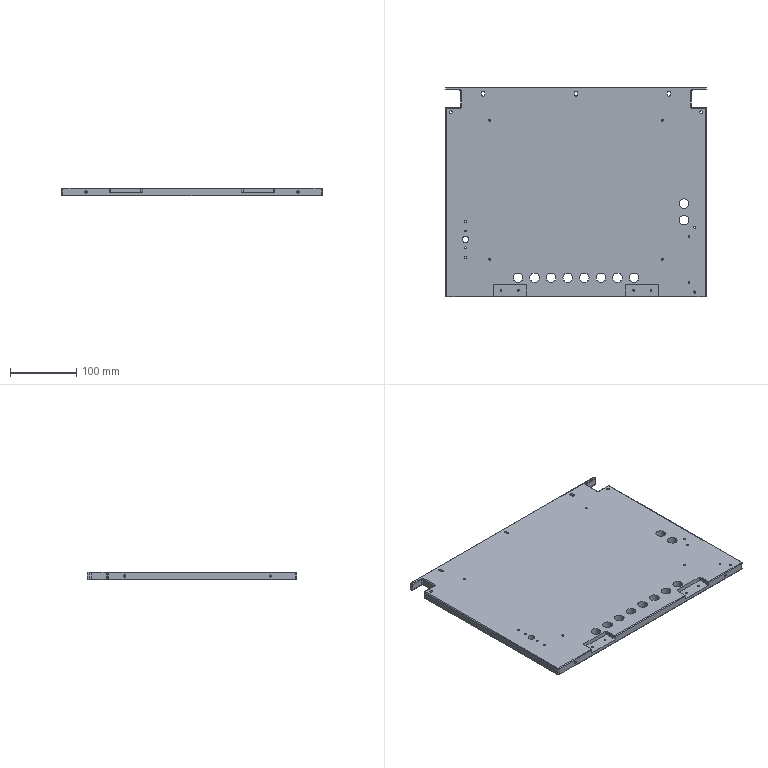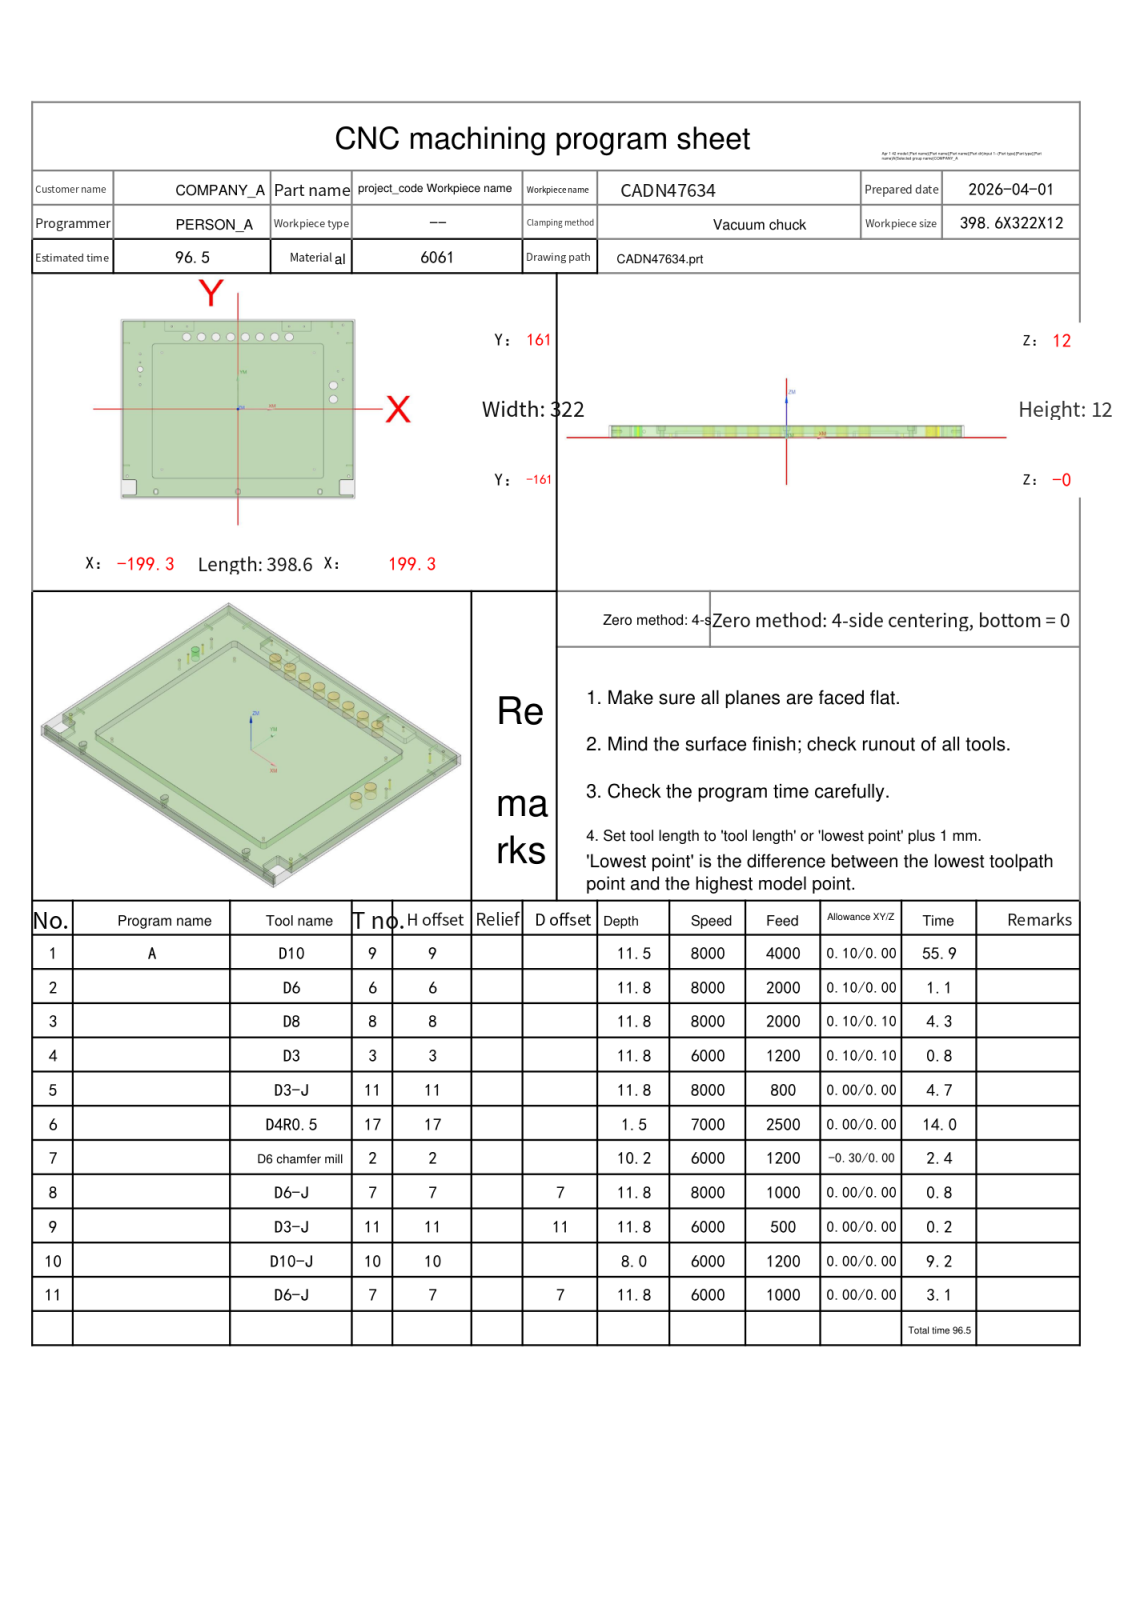NC program | NX | posted by the shop | part box 393.6 x 317 x 12 mm
Lines 3048 to 3819 of 16012:
N3 T08 M06
(D8  D=8. R=0. H=08 ce=0.10 di=0.10)
G00 G90 G54 X165.838 Y18.299 M03 S8000
G43 H08 Z32.
M08
Z13.
G01 X165.647 Y18.916 Z12.966 F2000.
X165.049 Y19.749 Z12.912
X164.216 Y20.347 Z12.859
X163.236 Y20.65 Z12.805
X162.364 Z12.759
X161.384 Y20.347 Z12.705
X160.551 Y19.749 Z12.652
X159.953 Y18.916 Z12.598
X159.65 Y17.936 Z12.544
Y17.5 Z12.521
Y17.064 Z12.499
X159.953 Y16.084 Z12.445
X160.551 Y15.251 Z12.391
X161.384 Y14.653 Z12.337
X162.364 Y14.35 Z12.284
X163.236 Z12.238
X164.216 Y14.653 Z12.184
X165.049 Y15.251 Z12.13
X165.647 Y16.084 Z12.077
X165.95 Y17.064 Z12.023
Y17.5 Z12.
G03 X162.8 Y20.65 Z11.926 I-3.15 J0.0
X159.65 Y17.5 Z11.853 I0.0 J-3.15
X162.8 Y14.35 Z11.779 I3.15 J0.0
X165.95 Y17.5 Z11.705 I0.0 J3.15
X162.8 Y20.65 Z11.631 I-3.15 J0.0
X159.65 Y17.5 Z11.558 I0.0 J-3.15
X162.8 Y14.35 Z11.484 I3.15 J0.0
X165.95 Y17.5 Z11.41 I0.0 J3.15
X162.8 Y20.65 Z11.336 I-3.15 J0.0
X159.65 Y17.5 Z11.263 I0.0 J-3.15
X162.8 Y14.35 Z11.189 I3.15 J0.0
X165.95 Y17.5 Z11.115 I0.0 J3.15
X162.8 Y20.65 Z11.041 I-3.15 J0.0
X159.65 Y17.5 Z10.968 I0.0 J-3.15
X162.8 Y14.35 Z10.894 I3.15 J0.0
X165.95 Y17.5 Z10.82 I0.0 J3.15
X162.8 Y20.65 Z10.746 I-3.15 J0.0
X159.65 Y17.5 Z10.673 I0.0 J-3.15
X162.8 Y14.35 Z10.599 I3.15 J0.0
X165.95 Y17.5 Z10.525 I0.0 J3.15
X162.8 Y20.65 Z10.451 I-3.15 J0.0
X159.65 Y17.5 Z10.378 I0.0 J-3.15
X162.8 Y14.35 Z10.304 I3.15 J0.0
X165.95 Y17.5 Z10.23 I0.0 J3.15
X162.8 Y20.65 Z10.156 I-3.15 J0.0
X159.65 Y17.5 Z10.083 I0.0 J-3.15
X162.8 Y14.35 Z10.009 I3.15 J0.0
X165.95 Y17.5 Z9.935 I0.0 J3.15
X162.8 Y20.65 Z9.861 I-3.15 J0.0
X159.65 Y17.5 Z9.788 I0.0 J-3.15
X162.8 Y14.35 Z9.714 I3.15 J0.0
X165.95 Y17.5 Z9.64 I0.0 J3.15
X162.8 Y20.65 Z9.566 I-3.15 J0.0
X159.65 Y17.5 Z9.493 I0.0 J-3.15
X162.8 Y14.35 Z9.419 I3.15 J0.0
X165.95 Y17.5 Z9.345 I0.0 J3.15
X162.8 Y20.65 Z9.271 I-3.15 J0.0
X159.65 Y17.5 Z9.198 I0.0 J-3.15
X162.8 Y14.35 Z9.124 I3.15 J0.0
X165.95 Y17.5 Z9.05 I0.0 J3.15
X162.8 Y20.65 Z8.976 I-3.15 J0.0
X159.65 Y17.5 Z8.903 I0.0 J-3.15
X162.8 Y14.35 Z8.829 I3.15 J0.0
X165.95 Y17.5 Z8.755 I0.0 J3.15
X162.8 Y20.65 Z8.681 I-3.15 J0.0
X159.65 Y17.5 Z8.608 I0.0 J-3.15
X162.8 Y14.35 Z8.534 I3.15 J0.0
X165.95 Y17.5 Z8.46 I0.0 J3.15
X162.8 Y20.65 Z8.386 I-3.15 J0.0
X159.65 Y17.5 Z8.313 I0.0 J-3.15
X162.8 Y14.35 Z8.239 I3.15 J0.0
X165.95 Y17.5 Z8.165 I0.0 J3.15
X162.8 Y20.65 Z8.091 I-3.15 J0.0
X159.65 Y17.5 Z8.018 I0.0 J-3.15
X162.8 Y14.35 Z7.944 I3.15 J0.0
X165.95 Y17.5 Z7.87 I0.0 J3.15
X162.8 Y20.65 Z7.796 I-3.15 J0.0
X159.65 Y17.5 Z7.723 I0.0 J-3.15
X162.8 Y14.35 Z7.649 I3.15 J0.0
X165.95 Y17.5 Z7.575 I0.0 J3.15
X162.8 Y20.65 Z7.501 I-3.15 J0.0
X159.65 Y17.5 Z7.428 I0.0 J-3.15
X162.8 Y14.35 Z7.354 I3.15 J0.0
X165.95 Y17.5 Z7.28 I0.0 J3.15
X162.8 Y20.65 Z7.206 I-3.15 J0.0
X159.65 Y17.5 Z7.133 I0.0 J-3.15
X162.8 Y14.35 Z7.059 I3.15 J0.0
X165.95 Y17.5 Z6.985 I0.0 J3.15
X162.8 Y20.65 Z6.911 I-3.15 J0.0
X159.65 Y17.5 Z6.838 I0.0 J-3.15
X162.8 Y14.35 Z6.764 I3.15 J0.0
X165.95 Y17.5 Z6.69 I0.0 J3.15
X162.8 Y20.65 Z6.616 I-3.15 J0.0
X159.65 Y17.5 Z6.543 I0.0 J-3.15
X162.8 Y14.35 Z6.469 I3.15 J0.0
X165.95 Y17.5 Z6.395 I0.0 J3.15
X162.8 Y20.65 Z6.321 I-3.15 J0.0
X159.65 Y17.5 Z6.248 I0.0 J-3.15
X162.8 Y14.35 Z6.174 I3.15 J0.0
X165.95 Y17.5 Z6.1 I0.0 J3.15
X162.8 Y20.65 Z6.026 I-3.15 J0.0
X159.65 Y17.5 Z5.953 I0.0 J-3.15
X162.8 Y14.35 Z5.879 I3.15 J0.0
X165.95 Y17.5 Z5.805 I0.0 J3.15
X162.8 Y20.65 Z5.731 I-3.15 J0.0
X159.65 Y17.5 Z5.658 I0.0 J-3.15
X162.8 Y14.35 Z5.584 I3.15 J0.0
X165.95 Y17.5 Z5.51 I0.0 J3.15
X162.8 Y20.65 Z5.436 I-3.15 J0.0
X159.65 Y17.5 Z5.363 I0.0 J-3.15
X162.8 Y14.35 Z5.289 I3.15 J0.0
X165.95 Y17.5 Z5.215 I0.0 J3.15
X162.8 Y20.65 Z5.141 I-3.15 J0.0
X159.65 Y17.5 Z5.068 I0.0 J-3.15
X162.8 Y14.35 Z4.994 I3.15 J0.0
X165.95 Y17.5 Z4.92 I0.0 J3.15
X162.8 Y20.65 Z4.846 I-3.15 J0.0
X159.65 Y17.5 Z4.773 I0.0 J-3.15
X162.8 Y14.35 Z4.699 I3.15 J0.0
X165.95 Y17.5 Z4.625 I0.0 J3.15
X162.8 Y20.65 Z4.551 I-3.15 J0.0
X159.65 Y17.5 Z4.478 I0.0 J-3.15
X162.8 Y14.35 Z4.404 I3.15 J0.0
X165.95 Y17.5 Z4.33 I0.0 J3.15
X162.8 Y20.65 Z4.256 I-3.15 J0.0
X159.65 Y17.5 Z4.183 I0.0 J-3.15
X162.8 Y14.35 Z4.109 I3.15 J0.0
X165.95 Y17.5 Z4.035 I0.0 J3.15
X162.8 Y20.65 Z3.961 I-3.15 J0.0
X159.65 Y17.5 Z3.888 I0.0 J-3.15
X162.8 Y14.35 Z3.814 I3.15 J0.0
X165.95 Y17.5 Z3.74 I0.0 J3.15
X162.8 Y20.65 Z3.666 I-3.15 J0.0
X159.65 Y17.5 Z3.593 I0.0 J-3.15
X162.8 Y14.35 Z3.519 I3.15 J0.0
X165.95 Y17.5 Z3.445 I0.0 J3.15
X162.8 Y20.65 Z3.371 I-3.15 J0.0
X159.65 Y17.5 Z3.298 I0.0 J-3.15
X162.8 Y14.35 Z3.224 I3.15 J0.0
X165.95 Y17.5 Z3.15 I0.0 J3.15
X162.8 Y20.65 Z3.076 I-3.15 J0.0
X159.65 Y17.5 Z3.003 I0.0 J-3.15
X162.8 Y14.35 Z2.929 I3.15 J0.0
X165.95 Y17.5 Z2.855 I0.0 J3.15
X162.8 Y20.65 Z2.781 I-3.15 J0.0
X159.65 Y17.5 Z2.708 I0.0 J-3.15
X162.8 Y14.35 Z2.634 I3.15 J0.0
X165.95 Y17.5 Z2.56 I0.0 J3.15
X162.8 Y20.65 Z2.486 I-3.15 J0.0
X159.65 Y17.5 Z2.413 I0.0 J-3.15
X162.8 Y14.35 Z2.339 I3.15 J0.0
X165.95 Y17.5 Z2.265 I0.0 J3.15
X162.8 Y20.65 Z2.191 I-3.15 J0.0
X159.65 Y17.5 Z2.118 I0.0 J-3.15
X162.8 Y14.35 Z2.044 I3.15 J0.0
X165.95 Y17.5 Z1.97 I0.0 J3.15
X162.8 Y20.65 Z1.896 I-3.15 J0.0
X159.65 Y17.5 Z1.823 I0.0 J-3.15
X162.8 Y14.35 Z1.749 I3.15 J0.0
X165.95 Y17.5 Z1.675 I0.0 J3.15
X162.8 Y20.65 Z1.601 I-3.15 J0.0
X159.65 Y17.5 Z1.528 I0.0 J-3.15
X162.8 Y14.35 Z1.454 I3.15 J0.0
X165.95 Y17.5 Z1.38 I0.0 J3.15
X162.8 Y20.65 Z1.306 I-3.15 J0.0
X159.65 Y17.5 Z1.233 I0.0 J-3.15
X162.8 Y14.35 Z1.159 I3.15 J0.0
X165.95 Y17.5 Z1.085 I0.0 J3.15
X162.8 Y20.65 Z1.011 I-3.15 J0.0
X159.65 Y17.5 Z.938 I0.0 J-3.15
X162.8 Y14.35 Z.864 I3.15 J0.0
X165.95 Y17.5 Z.79 I0.0 J3.15
X162.8 Y20.65 Z.716 I-3.15 J0.0
X159.65 Y17.5 Z.643 I0.0 J-3.15
X162.8 Y14.35 Z.569 I3.15 J0.0
X165.95 Y17.5 Z.495 I0.0 J3.15
X162.8 Y20.65 Z.421 I-3.15 J0.0
X159.65 Y17.5 Z.348 I0.0 J-3.15
X162.8 Y14.35 Z.274 I3.15 J0.0
X165.95 Y17.5 Z.2 I0.0 J3.15
X162.8 Y20.65 I-3.15 J0.0
X159.65 Y17.5 I0.0 J-3.15
X162.8 Y14.35 I3.15 J0.0
X165.95 Y17.5 I0.0 J3.15
X165.925 Y17.899 I-3.15 J0.0
G01 Z1.2
G00 Z32.
X165.838 Y43.299
Z13.
G01 X165.647 Y43.916 Z12.966
X165.049 Y44.749 Z12.912
X164.216 Y45.347 Z12.859
X163.236 Y45.65 Z12.805
X162.364 Z12.759
X161.384 Y45.347 Z12.705
X160.551 Y44.749 Z12.652
X159.953 Y43.916 Z12.598
X159.65 Y42.936 Z12.544
Y42.064 Z12.499
X159.953 Y41.084 Z12.445
X160.551 Y40.251 Z12.391
X161.384 Y39.653 Z12.337
X162.364 Y39.35 Z12.284
X163.236 Z12.238
X164.216 Y39.653 Z12.184
X165.049 Y40.251 Z12.13
X165.647 Y41.084 Z12.077
X165.95 Y42.064 Z12.023
Y42.5 Z12.
G03 X162.8 Y45.65 Z11.926 I-3.15 J0.0
X159.65 Y42.5 Z11.853 I0.0 J-3.15
X162.8 Y39.35 Z11.779 I3.15 J0.0
X165.95 Y42.5 Z11.705 I0.0 J3.15
X162.8 Y45.65 Z11.631 I-3.15 J0.0
X159.65 Y42.5 Z11.558 I0.0 J-3.15
X162.8 Y39.35 Z11.484 I3.15 J0.0
X165.95 Y42.5 Z11.41 I0.0 J3.15
X162.8 Y45.65 Z11.336 I-3.15 J0.0
X159.65 Y42.5 Z11.263 I0.0 J-3.15
X162.8 Y39.35 Z11.189 I3.15 J0.0
X165.95 Y42.5 Z11.115 I0.0 J3.15
X162.8 Y45.65 Z11.041 I-3.15 J0.0
X159.65 Y42.5 Z10.968 I0.0 J-3.15
X162.8 Y39.35 Z10.894 I3.15 J0.0
X165.95 Y42.5 Z10.82 I0.0 J3.15
X162.8 Y45.65 Z10.746 I-3.15 J0.0
X159.65 Y42.5 Z10.673 I0.0 J-3.15
X162.8 Y39.35 Z10.599 I3.15 J0.0
X165.95 Y42.5 Z10.525 I0.0 J3.15
X162.8 Y45.65 Z10.451 I-3.15 J0.0
X159.65 Y42.5 Z10.378 I0.0 J-3.15
X162.8 Y39.35 Z10.304 I3.15 J0.0
X165.95 Y42.5 Z10.23 I0.0 J3.15
X162.8 Y45.65 Z10.156 I-3.15 J0.0
X159.65 Y42.5 Z10.083 I0.0 J-3.15
X162.8 Y39.35 Z10.009 I3.15 J0.0
X165.95 Y42.5 Z9.935 I0.0 J3.15
X162.8 Y45.65 Z9.861 I-3.15 J0.0
X159.65 Y42.5 Z9.788 I0.0 J-3.15
X162.8 Y39.35 Z9.714 I3.15 J0.0
X165.95 Y42.5 Z9.64 I0.0 J3.15
X162.8 Y45.65 Z9.566 I-3.15 J0.0
X159.65 Y42.5 Z9.493 I0.0 J-3.15
X162.8 Y39.35 Z9.419 I3.15 J0.0
X165.95 Y42.5 Z9.345 I0.0 J3.15
X162.8 Y45.65 Z9.271 I-3.15 J0.0
X159.65 Y42.5 Z9.198 I0.0 J-3.15
X162.8 Y39.35 Z9.124 I3.15 J0.0
X165.95 Y42.5 Z9.05 I0.0 J3.15
X162.8 Y45.65 Z8.976 I-3.15 J0.0
X159.65 Y42.5 Z8.903 I0.0 J-3.15
X162.8 Y39.35 Z8.829 I3.15 J0.0
X165.95 Y42.5 Z8.755 I0.0 J3.15
X162.8 Y45.65 Z8.681 I-3.15 J0.0
X159.65 Y42.5 Z8.608 I0.0 J-3.15
X162.8 Y39.35 Z8.534 I3.15 J0.0
X165.95 Y42.5 Z8.46 I0.0 J3.15
X162.8 Y45.65 Z8.386 I-3.15 J0.0
X159.65 Y42.5 Z8.313 I0.0 J-3.15
X162.8 Y39.35 Z8.239 I3.15 J0.0
X165.95 Y42.5 Z8.165 I0.0 J3.15
X162.8 Y45.65 Z8.091 I-3.15 J0.0
X159.65 Y42.5 Z8.018 I0.0 J-3.15
X162.8 Y39.35 Z7.944 I3.15 J0.0
X165.95 Y42.5 Z7.87 I0.0 J3.15
X162.8 Y45.65 Z7.796 I-3.15 J0.0
X159.65 Y42.5 Z7.723 I0.0 J-3.15
X162.8 Y39.35 Z7.649 I3.15 J0.0
X165.95 Y42.5 Z7.575 I0.0 J3.15
X162.8 Y45.65 Z7.501 I-3.15 J0.0
X159.65 Y42.5 Z7.428 I0.0 J-3.15
X162.8 Y39.35 Z7.354 I3.15 J0.0
X165.95 Y42.5 Z7.28 I0.0 J3.15
X162.8 Y45.65 Z7.206 I-3.15 J0.0
X159.65 Y42.5 Z7.133 I0.0 J-3.15
X162.8 Y39.35 Z7.059 I3.15 J0.0
X165.95 Y42.5 Z6.985 I0.0 J3.15
X162.8 Y45.65 Z6.911 I-3.15 J0.0
X159.65 Y42.5 Z6.838 I0.0 J-3.15
X162.8 Y39.35 Z6.764 I3.15 J0.0
X165.95 Y42.5 Z6.69 I0.0 J3.15
X162.8 Y45.65 Z6.616 I-3.15 J0.0
X159.65 Y42.5 Z6.543 I0.0 J-3.15
X162.8 Y39.35 Z6.469 I3.15 J0.0
X165.95 Y42.5 Z6.395 I0.0 J3.15
X162.8 Y45.65 Z6.321 I-3.15 J0.0
X159.65 Y42.5 Z6.248 I0.0 J-3.15
X162.8 Y39.35 Z6.174 I3.15 J0.0
X165.95 Y42.5 Z6.1 I0.0 J3.15
X162.8 Y45.65 Z6.026 I-3.15 J0.0
X159.65 Y42.5 Z5.953 I0.0 J-3.15
X162.8 Y39.35 Z5.879 I3.15 J0.0
X165.95 Y42.5 Z5.805 I0.0 J3.15
X162.8 Y45.65 Z5.731 I-3.15 J0.0
X159.65 Y42.5 Z5.658 I0.0 J-3.15
X162.8 Y39.35 Z5.584 I3.15 J0.0
X165.95 Y42.5 Z5.51 I0.0 J3.15
X162.8 Y45.65 Z5.436 I-3.15 J0.0
X159.65 Y42.5 Z5.363 I0.0 J-3.15
X162.8 Y39.35 Z5.289 I3.15 J0.0
X165.95 Y42.5 Z5.215 I0.0 J3.15
X162.8 Y45.65 Z5.141 I-3.15 J0.0
X159.65 Y42.5 Z5.068 I0.0 J-3.15
X162.8 Y39.35 Z4.994 I3.15 J0.0
X165.95 Y42.5 Z4.92 I0.0 J3.15
X162.8 Y45.65 Z4.846 I-3.15 J0.0
X159.65 Y42.5 Z4.773 I0.0 J-3.15
X162.8 Y39.35 Z4.699 I3.15 J0.0
X165.95 Y42.5 Z4.625 I0.0 J3.15
X162.8 Y45.65 Z4.551 I-3.15 J0.0
X159.65 Y42.5 Z4.478 I0.0 J-3.15
X162.8 Y39.35 Z4.404 I3.15 J0.0
X165.95 Y42.5 Z4.33 I0.0 J3.15
X162.8 Y45.65 Z4.256 I-3.15 J0.0
X159.65 Y42.5 Z4.183 I0.0 J-3.15
X162.8 Y39.35 Z4.109 I3.15 J0.0
X165.95 Y42.5 Z4.035 I0.0 J3.15
X162.8 Y45.65 Z3.961 I-3.15 J0.0
X159.65 Y42.5 Z3.888 I0.0 J-3.15
X162.8 Y39.35 Z3.814 I3.15 J0.0
X165.95 Y42.5 Z3.74 I0.0 J3.15
X162.8 Y45.65 Z3.666 I-3.15 J0.0
X159.65 Y42.5 Z3.593 I0.0 J-3.15
X162.8 Y39.35 Z3.519 I3.15 J0.0
X165.95 Y42.5 Z3.445 I0.0 J3.15
X162.8 Y45.65 Z3.371 I-3.15 J0.0
X159.65 Y42.5 Z3.298 I0.0 J-3.15
X162.8 Y39.35 Z3.224 I3.15 J0.0
X165.95 Y42.5 Z3.15 I0.0 J3.15
X162.8 Y45.65 Z3.076 I-3.15 J0.0
X159.65 Y42.5 Z3.003 I0.0 J-3.15
X162.8 Y39.35 Z2.929 I3.15 J0.0
X165.95 Y42.5 Z2.855 I0.0 J3.15
X162.8 Y45.65 Z2.781 I-3.15 J0.0
X159.65 Y42.5 Z2.708 I0.0 J-3.15
X162.8 Y39.35 Z2.634 I3.15 J0.0
X165.95 Y42.5 Z2.56 I0.0 J3.15
X162.8 Y45.65 Z2.486 I-3.15 J0.0
X159.65 Y42.5 Z2.413 I0.0 J-3.15
X162.8 Y39.35 Z2.339 I3.15 J0.0
X165.95 Y42.5 Z2.265 I0.0 J3.15
X162.8 Y45.65 Z2.191 I-3.15 J0.0
X159.65 Y42.5 Z2.118 I0.0 J-3.15
X162.8 Y39.35 Z2.044 I3.15 J0.0
X165.95 Y42.5 Z1.97 I0.0 J3.15
X162.8 Y45.65 Z1.896 I-3.15 J0.0
X159.65 Y42.5 Z1.823 I0.0 J-3.15
X162.8 Y39.35 Z1.749 I3.15 J0.0
X165.95 Y42.5 Z1.675 I0.0 J3.15
X162.8 Y45.65 Z1.601 I-3.15 J0.0
X159.65 Y42.5 Z1.528 I0.0 J-3.15
X162.8 Y39.35 Z1.454 I3.15 J0.0
X165.95 Y42.5 Z1.38 I0.0 J3.15
X162.8 Y45.65 Z1.306 I-3.15 J0.0
X159.65 Y42.5 Z1.233 I0.0 J-3.15
X162.8 Y39.35 Z1.159 I3.15 J0.0
X165.95 Y42.5 Z1.085 I0.0 J3.15
X162.8 Y45.65 Z1.011 I-3.15 J0.0
X159.65 Y42.5 Z.938 I0.0 J-3.15
X162.8 Y39.35 Z.864 I3.15 J0.0
X165.95 Y42.5 Z.79 I0.0 J3.15
X162.8 Y45.65 Z.716 I-3.15 J0.0
X159.65 Y42.5 Z.643 I0.0 J-3.15
X162.8 Y39.35 Z.569 I3.15 J0.0
X165.95 Y42.5 Z.495 I0.0 J3.15
X162.8 Y45.65 Z.421 I-3.15 J0.0
X159.65 Y42.5 Z.348 I0.0 J-3.15
X162.8 Y39.35 Z.274 I3.15 J0.0
X165.95 Y42.5 Z.2 I0.0 J3.15
X162.8 Y45.65 I-3.15 J0.0
X159.65 Y42.5 I0.0 J-3.15
X162.8 Y39.35 I3.15 J0.0
X165.95 Y42.5 I0.0 J3.15
X165.925 Y42.899 I-3.15 J0.0
G01 Z1.2
G00 Z32.
X-88.299 Y132.538
Z13.
G01 X-88.916 Y132.347 Z12.966
X-89.749 Y131.749 Z12.912
X-90.347 Y130.916 Z12.859
X-90.65 Y129.936 Z12.805
Y129.5 Z12.782
Y129.064 Z12.759
X-90.347 Y128.084 Z12.705
X-89.749 Y127.251 Z12.652
X-88.916 Y126.653 Z12.598
X-87.936 Y126.35 Z12.544
X-87.064 Z12.499
X-86.084 Y126.653 Z12.445
X-85.251 Y127.251 Z12.391
X-84.653 Y128.084 Z12.337
X-84.35 Y129.064 Z12.284
Y129.936 Z12.238
X-84.653 Y130.916 Z12.184
X-85.251 Y131.749 Z12.13
X-86.084 Y132.347 Z12.077
X-87.064 Y132.65 Z12.023
X-87.5 Z12.
G03 X-90.65 Y129.5 Z11.926 I0.0 J-3.15
X-87.5 Y126.35 Z11.853 I3.15 J0.0
X-84.35 Y129.5 Z11.779 I0.0 J3.15
X-87.5 Y132.65 Z11.705 I-3.15 J0.0
X-90.65 Y129.5 Z11.631 I0.0 J-3.15
X-87.5 Y126.35 Z11.558 I3.15 J0.0
X-84.35 Y129.5 Z11.484 I0.0 J3.15
X-87.5 Y132.65 Z11.41 I-3.15 J0.0
X-90.65 Y129.5 Z11.336 I0.0 J-3.15
X-87.5 Y126.35 Z11.263 I3.15 J0.0
X-84.35 Y129.5 Z11.189 I0.0 J3.15
X-87.5 Y132.65 Z11.115 I-3.15 J0.0
X-90.65 Y129.5 Z11.041 I0.0 J-3.15
X-87.5 Y126.35 Z10.968 I3.15 J0.0
X-84.35 Y129.5 Z10.894 I0.0 J3.15
X-87.5 Y132.65 Z10.82 I-3.15 J0.0
X-90.65 Y129.5 Z10.746 I0.0 J-3.15
X-87.5 Y126.35 Z10.673 I3.15 J0.0
X-84.35 Y129.5 Z10.599 I0.0 J3.15
X-87.5 Y132.65 Z10.525 I-3.15 J0.0
X-90.65 Y129.5 Z10.451 I0.0 J-3.15
X-87.5 Y126.35 Z10.378 I3.15 J0.0
X-84.35 Y129.5 Z10.304 I0.0 J3.15
X-87.5 Y132.65 Z10.23 I-3.15 J0.0
X-90.65 Y129.5 Z10.156 I0.0 J-3.15
X-87.5 Y126.35 Z10.083 I3.15 J0.0
X-84.35 Y129.5 Z10.009 I0.0 J3.15
X-87.5 Y132.65 Z9.935 I-3.15 J0.0
X-90.65 Y129.5 Z9.861 I0.0 J-3.15
X-87.5 Y126.35 Z9.788 I3.15 J0.0
X-84.35 Y129.5 Z9.714 I0.0 J3.15
X-87.5 Y132.65 Z9.64 I-3.15 J0.0
X-90.65 Y129.5 Z9.566 I0.0 J-3.15
X-87.5 Y126.35 Z9.493 I3.15 J0.0
X-84.35 Y129.5 Z9.419 I0.0 J3.15
X-87.5 Y132.65 Z9.345 I-3.15 J0.0
X-90.65 Y129.5 Z9.271 I0.0 J-3.15
X-87.5 Y126.35 Z9.198 I3.15 J0.0
X-84.35 Y129.5 Z9.124 I0.0 J3.15
X-87.5 Y132.65 Z9.05 I-3.15 J0.0
X-90.65 Y129.5 Z8.976 I0.0 J-3.15
X-87.5 Y126.35 Z8.903 I3.15 J0.0
X-84.35 Y129.5 Z8.829 I0.0 J3.15
X-87.5 Y132.65 Z8.755 I-3.15 J0.0
X-90.65 Y129.5 Z8.681 I0.0 J-3.15
X-87.5 Y126.35 Z8.608 I3.15 J0.0
X-84.35 Y129.5 Z8.534 I0.0 J3.15
X-87.5 Y132.65 Z8.46 I-3.15 J0.0
X-90.65 Y129.5 Z8.386 I0.0 J-3.15
X-87.5 Y126.35 Z8.313 I3.15 J0.0
X-84.35 Y129.5 Z8.239 I0.0 J3.15
X-87.5 Y132.65 Z8.165 I-3.15 J0.0
X-90.65 Y129.5 Z8.091 I0.0 J-3.15
X-87.5 Y126.35 Z8.018 I3.15 J0.0
X-84.35 Y129.5 Z7.944 I0.0 J3.15
X-87.5 Y132.65 Z7.87 I-3.15 J0.0
X-90.65 Y129.5 Z7.796 I0.0 J-3.15
X-87.5 Y126.35 Z7.723 I3.15 J0.0
X-84.35 Y129.5 Z7.649 I0.0 J3.15
X-87.5 Y132.65 Z7.575 I-3.15 J0.0
X-90.65 Y129.5 Z7.501 I0.0 J-3.15
X-87.5 Y126.35 Z7.428 I3.15 J0.0
X-84.35 Y129.5 Z7.354 I0.0 J3.15
X-87.5 Y132.65 Z7.28 I-3.15 J0.0
X-90.65 Y129.5 Z7.206 I0.0 J-3.15
X-87.5 Y126.35 Z7.133 I3.15 J0.0
X-84.35 Y129.5 Z7.059 I0.0 J3.15
X-87.5 Y132.65 Z6.985 I-3.15 J0.0
X-90.65 Y129.5 Z6.911 I0.0 J-3.15
X-87.5 Y126.35 Z6.838 I3.15 J0.0
X-84.35 Y129.5 Z6.764 I0.0 J3.15
X-87.5 Y132.65 Z6.69 I-3.15 J0.0
X-90.65 Y129.5 Z6.616 I0.0 J-3.15
X-87.5 Y126.35 Z6.543 I3.15 J0.0
X-84.35 Y129.5 Z6.469 I0.0 J3.15
X-87.5 Y132.65 Z6.395 I-3.15 J0.0
X-90.65 Y129.5 Z6.321 I0.0 J-3.15
X-87.5 Y126.35 Z6.248 I3.15 J0.0
X-84.35 Y129.5 Z6.174 I0.0 J3.15
X-87.5 Y132.65 Z6.1 I-3.15 J0.0
X-90.65 Y129.5 Z6.026 I0.0 J-3.15
X-87.5 Y126.35 Z5.953 I3.15 J0.0
X-84.35 Y129.5 Z5.879 I0.0 J3.15
X-87.5 Y132.65 Z5.805 I-3.15 J0.0
X-90.65 Y129.5 Z5.731 I0.0 J-3.15
X-87.5 Y126.35 Z5.658 I3.15 J0.0
X-84.35 Y129.5 Z5.584 I0.0 J3.15
X-87.5 Y132.65 Z5.51 I-3.15 J0.0
X-90.65 Y129.5 Z5.436 I0.0 J-3.15
X-87.5 Y126.35 Z5.363 I3.15 J0.0
X-84.35 Y129.5 Z5.289 I0.0 J3.15
X-87.5 Y132.65 Z5.215 I-3.15 J0.0
X-90.65 Y129.5 Z5.141 I0.0 J-3.15
X-87.5 Y126.35 Z5.068 I3.15 J0.0
X-84.35 Y129.5 Z4.994 I0.0 J3.15
X-87.5 Y132.65 Z4.92 I-3.15 J0.0
X-90.65 Y129.5 Z4.846 I0.0 J-3.15
X-87.5 Y126.35 Z4.773 I3.15 J0.0
X-84.35 Y129.5 Z4.699 I0.0 J3.15
X-87.5 Y132.65 Z4.625 I-3.15 J0.0
X-90.65 Y129.5 Z4.551 I0.0 J-3.15
X-87.5 Y126.35 Z4.478 I3.15 J0.0
X-84.35 Y129.5 Z4.404 I0.0 J3.15
X-87.5 Y132.65 Z4.33 I-3.15 J0.0
X-90.65 Y129.5 Z4.256 I0.0 J-3.15
X-87.5 Y126.35 Z4.183 I3.15 J0.0
X-84.35 Y129.5 Z4.109 I0.0 J3.15
X-87.5 Y132.65 Z4.035 I-3.15 J0.0
X-90.65 Y129.5 Z3.961 I0.0 J-3.15
X-87.5 Y126.35 Z3.888 I3.15 J0.0
X-84.35 Y129.5 Z3.814 I0.0 J3.15
X-87.5 Y132.65 Z3.74 I-3.15 J0.0
X-90.65 Y129.5 Z3.666 I0.0 J-3.15
X-87.5 Y126.35 Z3.593 I3.15 J0.0
X-84.35 Y129.5 Z3.519 I0.0 J3.15
X-87.5 Y132.65 Z3.445 I-3.15 J0.0
X-90.65 Y129.5 Z3.371 I0.0 J-3.15
X-87.5 Y126.35 Z3.298 I3.15 J0.0
X-84.35 Y129.5 Z3.224 I0.0 J3.15
X-87.5 Y132.65 Z3.15 I-3.15 J0.0
X-90.65 Y129.5 Z3.076 I0.0 J-3.15
X-87.5 Y126.35 Z3.003 I3.15 J0.0
X-84.35 Y129.5 Z2.929 I0.0 J3.15
X-87.5 Y132.65 Z2.855 I-3.15 J0.0
X-90.65 Y129.5 Z2.781 I0.0 J-3.15
X-87.5 Y126.35 Z2.708 I3.15 J0.0
X-84.35 Y129.5 Z2.634 I0.0 J3.15
X-87.5 Y132.65 Z2.56 I-3.15 J0.0
X-90.65 Y129.5 Z2.486 I0.0 J-3.15
X-87.5 Y126.35 Z2.413 I3.15 J0.0
X-84.35 Y129.5 Z2.339 I0.0 J3.15
X-87.5 Y132.65 Z2.265 I-3.15 J0.0
X-90.65 Y129.5 Z2.191 I0.0 J-3.15
X-87.5 Y126.35 Z2.118 I3.15 J0.0
X-84.35 Y129.5 Z2.044 I0.0 J3.15
X-87.5 Y132.65 Z1.97 I-3.15 J0.0
X-90.65 Y129.5 Z1.896 I0.0 J-3.15
X-87.5 Y126.35 Z1.823 I3.15 J0.0
X-84.35 Y129.5 Z1.749 I0.0 J3.15
X-87.5 Y132.65 Z1.675 I-3.15 J0.0
X-90.65 Y129.5 Z1.601 I0.0 J-3.15
X-87.5 Y126.35 Z1.528 I3.15 J0.0
X-84.35 Y129.5 Z1.454 I0.0 J3.15
X-87.5 Y132.65 Z1.38 I-3.15 J0.0
X-90.65 Y129.5 Z1.306 I0.0 J-3.15
X-87.5 Y126.35 Z1.233 I3.15 J0.0
X-84.35 Y129.5 Z1.159 I0.0 J3.15
X-87.5 Y132.65 Z1.085 I-3.15 J0.0
X-90.65 Y129.5 Z1.011 I0.0 J-3.15
X-87.5 Y126.35 Z.938 I3.15 J0.0
X-84.35 Y129.5 Z.864 I0.0 J3.15
X-87.5 Y132.65 Z.79 I-3.15 J0.0
X-90.65 Y129.5 Z.716 I0.0 J-3.15
X-87.5 Y126.35 Z.643 I3.15 J0.0
X-84.35 Y129.5 Z.569 I0.0 J3.15
X-87.5 Y132.65 Z.495 I-3.15 J0.0
X-90.65 Y129.5 Z.421 I0.0 J-3.15
X-87.5 Y126.35 Z.348 I3.15 J0.0
X-84.35 Y129.5 Z.274 I0.0 J3.15
X-87.5 Y132.65 Z.2 I-3.15 J0.0
X-90.65 Y129.5 I0.0 J-3.15
X-87.5 Y126.35 I3.15 J0.0
X-84.35 Y129.5 I0.0 J3.15
X-87.5 Y132.65 I-3.15 J0.0
X-87.899 Y132.625 I0.0 J-3.15
G01 Z1.2
G00 Z32.
X-63.299 Y132.538
Z13.
G01 X-63.916 Y132.347 Z12.966
X-64.749 Y131.749 Z12.912
X-65.347 Y130.916 Z12.859
X-65.65 Y129.936 Z12.805
Y129.5 Z12.782
Y129.064 Z12.759
X-65.347 Y128.084 Z12.705
X-64.749 Y127.251 Z12.652
X-63.916 Y126.653 Z12.598
X-62.936 Y126.35 Z12.544
X-62.5 Z12.521
X-62.064 Z12.499
X-61.084 Y126.653 Z12.445
X-60.251 Y127.251 Z12.391
X-59.653 Y128.084 Z12.337
X-59.35 Y129.064 Z12.284
Y129.5 Z12.261
Y129.936 Z12.238
X-59.653 Y130.916 Z12.184
X-60.251 Y131.749 Z12.13
X-61.084 Y132.347 Z12.077
X-62.064 Y132.65 Z12.023
X-62.5 Z12.
G03 X-65.65 Y129.5 Z11.926 I0.0 J-3.15
X-62.5 Y126.35 Z11.853 I3.15 J0.0
X-59.35 Y129.5 Z11.779 I0.0 J3.15
X-62.5 Y132.65 Z11.705 I-3.15 J0.0
X-65.65 Y129.5 Z11.631 I0.0 J-3.15
X-62.5 Y126.35 Z11.558 I3.15 J0.0
X-59.35 Y129.5 Z11.484 I0.0 J3.15
X-62.5 Y132.65 Z11.41 I-3.15 J0.0
X-65.65 Y129.5 Z11.336 I0.0 J-3.15
X-62.5 Y126.35 Z11.263 I3.15 J0.0
X-59.35 Y129.5 Z11.189 I0.0 J3.15
X-62.5 Y132.65 Z11.115 I-3.15 J0.0
X-65.65 Y129.5 Z11.041 I0.0 J-3.15
X-62.5 Y126.35 Z10.968 I3.15 J0.0
X-59.35 Y129.5 Z10.894 I0.0 J3.15
X-62.5 Y132.65 Z10.82 I-3.15 J0.0
X-65.65 Y129.5 Z10.746 I0.0 J-3.15
X-62.5 Y126.35 Z10.673 I3.15 J0.0
X-59.35 Y129.5 Z10.599 I0.0 J3.15
X-62.5 Y132.65 Z10.525 I-3.15 J0.0
X-65.65 Y129.5 Z10.451 I0.0 J-3.15
X-62.5 Y126.35 Z10.378 I3.15 J0.0
X-59.35 Y129.5 Z10.304 I0.0 J3.15
X-62.5 Y132.65 Z10.23 I-3.15 J0.0
X-65.65 Y129.5 Z10.156 I0.0 J-3.15
X-62.5 Y126.35 Z10.083 I3.15 J0.0
X-59.35 Y129.5 Z10.009 I0.0 J3.15
X-62.5 Y132.65 Z9.935 I-3.15 J0.0
X-65.65 Y129.5 Z9.861 I0.0 J-3.15
X-62.5 Y126.35 Z9.788 I3.15 J0.0
X-59.35 Y129.5 Z9.714 I0.0 J3.15
X-62.5 Y132.65 Z9.64 I-3.15 J0.0
X-65.65 Y129.5 Z9.566 I0.0 J-3.15
X-62.5 Y126.35 Z9.493 I3.15 J0.0
X-59.35 Y129.5 Z9.419 I0.0 J3.15
X-62.5 Y132.65 Z9.345 I-3.15 J0.0
X-65.65 Y129.5 Z9.271 I0.0 J-3.15
X-62.5 Y126.35 Z9.198 I3.15 J0.0
X-59.35 Y129.5 Z9.124 I0.0 J3.15
X-62.5 Y132.65 Z9.05 I-3.15 J0.0
X-65.65 Y129.5 Z8.976 I0.0 J-3.15
X-62.5 Y126.35 Z8.903 I3.15 J0.0
X-59.35 Y129.5 Z8.829 I0.0 J3.15
X-62.5 Y132.65 Z8.755 I-3.15 J0.0
X-65.65 Y129.5 Z8.681 I0.0 J-3.15
X-62.5 Y126.35 Z8.608 I3.15 J0.0
X-59.35 Y129.5 Z8.534 I0.0 J3.15
X-62.5 Y132.65 Z8.46 I-3.15 J0.0
X-65.65 Y129.5 Z8.386 I0.0 J-3.15
X-62.5 Y126.35 Z8.313 I3.15 J0.0
X-59.35 Y129.5 Z8.239 I0.0 J3.15
X-62.5 Y132.65 Z8.165 I-3.15 J0.0
X-65.65 Y129.5 Z8.091 I0.0 J-3.15
X-62.5 Y126.35 Z8.018 I3.15 J0.0
X-59.35 Y129.5 Z7.944 I0.0 J3.15
X-62.5 Y132.65 Z7.87 I-3.15 J0.0
X-65.65 Y129.5 Z7.796 I0.0 J-3.15
X-62.5 Y126.35 Z7.723 I3.15 J0.0
X-59.35 Y129.5 Z7.649 I0.0 J3.15
X-62.5 Y132.65 Z7.575 I-3.15 J0.0
X-65.65 Y129.5 Z7.501 I0.0 J-3.15
X-62.5 Y126.35 Z7.428 I3.15 J0.0
X-59.35 Y129.5 Z7.354 I0.0 J3.15
X-62.5 Y132.65 Z7.28 I-3.15 J0.0
X-65.65 Y129.5 Z7.206 I0.0 J-3.15
X-62.5 Y126.35 Z7.133 I3.15 J0.0
X-59.35 Y129.5 Z7.059 I0.0 J3.15
X-62.5 Y132.65 Z6.985 I-3.15 J0.0
X-65.65 Y129.5 Z6.911 I0.0 J-3.15
X-62.5 Y126.35 Z6.838 I3.15 J0.0
X-59.35 Y129.5 Z6.764 I0.0 J3.15
X-62.5 Y132.65 Z6.69 I-3.15 J0.0
X-65.65 Y129.5 Z6.616 I0.0 J-3.15
X-62.5 Y126.35 Z6.543 I3.15 J0.0
X-59.35 Y129.5 Z6.469 I0.0 J3.15
X-62.5 Y132.65 Z6.395 I-3.15 J0.0
X-65.65 Y129.5 Z6.321 I0.0 J-3.15
X-62.5 Y126.35 Z6.248 I3.15 J0.0
X-59.35 Y129.5 Z6.174 I0.0 J3.15
X-62.5 Y132.65 Z6.1 I-3.15 J0.0
X-65.65 Y129.5 Z6.026 I0.0 J-3.15
X-62.5 Y126.35 Z5.953 I3.15 J0.0
X-59.35 Y129.5 Z5.879 I0.0 J3.15
X-62.5 Y132.65 Z5.805 I-3.15 J0.0
X-65.65 Y129.5 Z5.731 I0.0 J-3.15
X-62.5 Y126.35 Z5.658 I3.15 J0.0
X-59.35 Y129.5 Z5.584 I0.0 J3.15
X-62.5 Y132.65 Z5.51 I-3.15 J0.0
X-65.65 Y129.5 Z5.436 I0.0 J-3.15
X-62.5 Y126.35 Z5.363 I3.15 J0.0
X-59.35 Y129.5 Z5.289 I0.0 J3.15
X-62.5 Y132.65 Z5.215 I-3.15 J0.0
X-65.65 Y129.5 Z5.141 I0.0 J-3.15
X-62.5 Y126.35 Z5.068 I3.15 J0.0
X-59.35 Y129.5 Z4.994 I0.0 J3.15
X-62.5 Y132.65 Z4.92 I-3.15 J0.0
X-65.65 Y129.5 Z4.846 I0.0 J-3.15
X-62.5 Y126.35 Z4.773 I3.15 J0.0
X-59.35 Y129.5 Z4.699 I0.0 J3.15
X-62.5 Y132.65 Z4.625 I-3.15 J0.0
X-65.65 Y129.5 Z4.551 I0.0 J-3.15
X-62.5 Y126.35 Z4.478 I3.15 J0.0
X-59.35 Y129.5 Z4.404 I0.0 J3.15
X-62.5 Y132.65 Z4.33 I-3.15 J0.0
X-65.65 Y129.5 Z4.256 I0.0 J-3.15
X-62.5 Y126.35 Z4.183 I3.15 J0.0
X-59.35 Y129.5 Z4.109 I0.0 J3.15
X-62.5 Y132.65 Z4.035 I-3.15 J0.0
X-65.65 Y129.5 Z3.961 I0.0 J-3.15
X-62.5 Y126.35 Z3.888 I3.15 J0.0
X-59.35 Y129.5 Z3.814 I0.0 J3.15
X-62.5 Y132.65 Z3.74 I-3.15 J0.0
X-65.65 Y129.5 Z3.666 I0.0 J-3.15
X-62.5 Y126.35 Z3.593 I3.15 J0.0
X-59.35 Y129.5 Z3.519 I0.0 J3.15
X-62.5 Y132.65 Z3.445 I-3.15 J0.0
X-65.65 Y129.5 Z3.371 I0.0 J-3.15
X-62.5 Y126.35 Z3.298 I3.15 J0.0
X-59.35 Y129.5 Z3.224 I0.0 J3.15
X-62.5 Y132.65 Z3.15 I-3.15 J0.0
X-65.65 Y129.5 Z3.076 I0.0 J-3.15
X-62.5 Y126.35 Z3.003 I3.15 J0.0
X-59.35 Y129.5 Z2.929 I0.0 J3.15
X-62.5 Y132.65 Z2.855 I-3.15 J0.0
X-65.65 Y129.5 Z2.781 I0.0 J-3.15
X-62.5 Y126.35 Z2.708 I3.15 J0.0
X-59.35 Y129.5 Z2.634 I0.0 J3.15
X-62.5 Y132.65 Z2.56 I-3.15 J0.0
X-65.65 Y129.5 Z2.486 I0.0 J-3.15
X-62.5 Y126.35 Z2.413 I3.15 J0.0
X-59.35 Y129.5 Z2.339 I0.0 J3.15
X-62.5 Y132.65 Z2.265 I-3.15 J0.0
X-65.65 Y129.5 Z2.191 I0.0 J-3.15
X-62.5 Y126.35 Z2.118 I3.15 J0.0
X-59.35 Y129.5 Z2.044 I0.0 J3.15
X-62.5 Y132.65 Z1.97 I-3.15 J0.0
X-65.65 Y129.5 Z1.896 I0.0 J-3.15
X-62.5 Y126.35 Z1.823 I3.15 J0.0
X-59.35 Y129.5 Z1.749 I0.0 J3.15
X-62.5 Y132.65 Z1.675 I-3.15 J0.0
X-65.65 Y129.5 Z1.601 I0.0 J-3.15
X-62.5 Y126.35 Z1.528 I3.15 J0.0
X-59.35 Y129.5 Z1.454 I0.0 J3.15
X-62.5 Y132.65 Z1.38 I-3.15 J0.0
X-65.65 Y129.5 Z1.306 I0.0 J-3.15
X-62.5 Y126.35 Z1.233 I3.15 J0.0
X-59.35 Y129.5 Z1.159 I0.0 J3.15
X-62.5 Y132.65 Z1.085 I-3.15 J0.0
X-65.65 Y129.5 Z1.011 I0.0 J-3.15
X-62.5 Y126.35 Z.938 I3.15 J0.0
X-59.35 Y129.5 Z.864 I0.0 J3.15
X-62.5 Y132.65 Z.79 I-3.15 J0.0
X-65.65 Y129.5 Z.716 I0.0 J-3.15
X-62.5 Y126.35 Z.643 I3.15 J0.0
X-59.35 Y129.5 Z.569 I0.0 J3.15
X-62.5 Y132.65 Z.495 I-3.15 J0.0
X-65.65 Y129.5 Z.421 I0.0 J-3.15
X-62.5 Y126.35 Z.348 I3.15 J0.0
X-59.35 Y129.5 Z.274 I0.0 J3.15
X-62.5 Y132.65 Z.2 I-3.15 J0.0
X-65.65 Y129.5 I0.0 J-3.15
X-62.5 Y126.35 I3.15 J0.0
X-59.35 Y129.5 I0.0 J3.15
X-62.5 Y132.65 I-3.15 J0.0
X-62.899 Y132.625 I0.0 J-3.15
G01 Z1.2
G00 Z32.
X-38.299 Y132.538
Z13.
G01 X-38.916 Y132.347 Z12.966
X-39.749 Y131.749 Z12.912
X-40.347 Y130.916 Z12.859
X-40.65 Y129.936 Z12.805
Y129.5 Z12.782